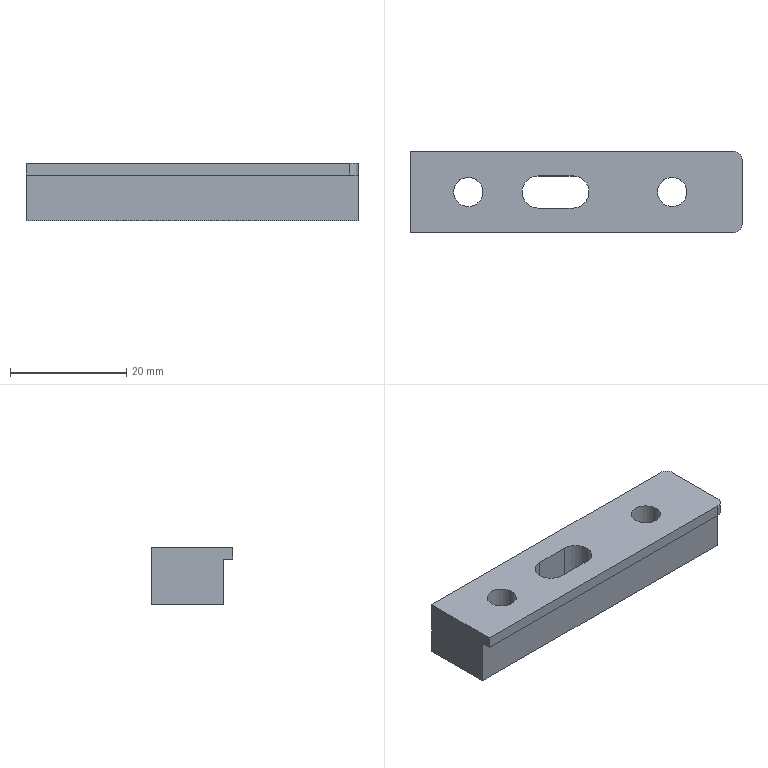Part | STEP file | 200 mesh_id6_xmt_t | 1 solid | 16 faces | box 57 x 14 x 9.8 mm | volume 6159 mm3 | plane 10 | cylinder 6 | commonest cylinder face diameters 3 x2 5.02 x2 5.5 x2
STEP:
#1=CARTESIAN_POINT('',(-16856.158,-3972.269,52.7));
#2=VERTEX_POINT('',#1);
#3=CARTESIAN_POINT('',(-16853.648,-3972.269,52.7));
#4=DIRECTION('',(0.,0.,-1.));
#5=DIRECTION('',(-1.,0.,0.));
#6=AXIS2_PLACEMENT_3D('',#3,#4,#5);
#7=CIRCLE('',#6,2.51);
#8=EDGE_CURVE('',#2,#2,#7,.T.);
#9=ORIENTED_EDGE('',*,*,#8,.T.);
#10=EDGE_LOOP('',(#9));
#11=FACE_BOUND('',#10,.T.);
#12=CARTESIAN_POINT('',(-16891.158,-3972.269,52.7));
#13=VERTEX_POINT('',#12);
#14=CARTESIAN_POINT('',(-16888.648,-3972.269,52.7));
#15=DIRECTION('',(0.,0.,-1.));
#16=DIRECTION('',(-1.,0.,0.));
#17=AXIS2_PLACEMENT_3D('',#14,#15,#16);
#18=CIRCLE('',#17,2.51);
#19=EDGE_CURVE('',#13,#13,#18,.T.);
#20=ORIENTED_EDGE('',*,*,#19,.T.);
#21=EDGE_LOOP('',(#20));
#22=FACE_BOUND('',#21,.T.);
#23=CARTESIAN_POINT('',(-16898.648,-3965.269,52.7));
#24=VERTEX_POINT('',#23);
#25=CARTESIAN_POINT('',(-16843.148,-3965.269,52.7));
#26=VERTEX_POINT('',#25);
#27=CARTESIAN_POINT('',(-16897.148,-3965.269,52.7));
#28=DIRECTION('',(1.,0.,0.));
#29=VECTOR('',#28,1.);
#30=LINE('',#27,#29);
#31=EDGE_CURVE('',#24,#26,#30,.T.);
#32=ORIENTED_EDGE('',*,*,#31,.F.);
#33=CARTESIAN_POINT('',(-16898.648,-3979.269,52.7));
#34=VERTEX_POINT('',#33);
#35=CARTESIAN_POINT('',(-16898.648,-3977.769,52.7));
#36=DIRECTION('',(0.,1.,0.));
#37=VECTOR('',#36,1.);
#38=LINE('',#35,#37);
#39=EDGE_CURVE('',#34,#24,#38,.T.);
#40=ORIENTED_EDGE('',*,*,#39,.F.);
#41=CARTESIAN_POINT('',(-16843.148,-3979.269,52.7));
#42=VERTEX_POINT('',#41);
#43=CARTESIAN_POINT('',(-16843.148,-3979.269,52.7));
#44=DIRECTION('',(-1.,0.,0.));
#45=VECTOR('',#44,1.);
#46=LINE('',#43,#45);
#47=EDGE_CURVE('',#42,#34,#46,.T.);
#48=ORIENTED_EDGE('',*,*,#47,.F.);
#49=CARTESIAN_POINT('',(-16841.648,-3977.769,52.7));
#50=VERTEX_POINT('',#49);
#51=CARTESIAN_POINT('',(-16843.148,-3977.769,52.7));
#52=DIRECTION('',(0.,0.,-1.));
#53=DIRECTION('',(1.,0.,0.));
#54=AXIS2_PLACEMENT_3D('',#51,#52,#53);
#55=CIRCLE('',#54,1.5);
#56=EDGE_CURVE('',#50,#42,#55,.T.);
#57=ORIENTED_EDGE('',*,*,#56,.F.);
#58=CARTESIAN_POINT('',(-16841.648,-3966.769,52.7));
#59=VERTEX_POINT('',#58);
#60=CARTESIAN_POINT('',(-16841.648,-3968.769,52.7));
#61=DIRECTION('',(0.,-1.,0.));
#62=VECTOR('',#61,1.);
#63=LINE('',#60,#62);
#64=EDGE_CURVE('',#59,#50,#63,.T.);
#65=ORIENTED_EDGE('',*,*,#64,.F.);
#66=CARTESIAN_POINT('',(-16843.148,-3966.769,52.7));
#67=DIRECTION('',(0.,0.,-1.));
#68=DIRECTION('',(-1.,0.,0.));
#69=AXIS2_PLACEMENT_3D('',#66,#67,#68);
#70=CIRCLE('',#69,1.5);
#71=EDGE_CURVE('',#26,#59,#70,.T.);
#72=ORIENTED_EDGE('',*,*,#71,.F.);
#73=EDGE_LOOP('',(#32,#40,#48,#57,#65,#72));
#74=FACE_BOUND('',#73,.T.);
#75=CARTESIAN_POINT('',(-16876.648,-3975.019,52.7));
#76=VERTEX_POINT('',#75);
#77=CARTESIAN_POINT('',(-16870.648,-3975.019,52.7));
#78=VERTEX_POINT('',#77);
#79=CARTESIAN_POINT('',(-16873.648,-3975.019,52.7));
#80=DIRECTION('',(1.,0.,0.));
#81=VECTOR('',#80,1.);
#82=LINE('',#79,#81);
#83=EDGE_CURVE('',#76,#78,#82,.T.);
#84=ORIENTED_EDGE('',*,*,#83,.F.);
#85=CARTESIAN_POINT('',(-16876.648,-3969.519,52.7));
#86=VERTEX_POINT('',#85);
#87=CARTESIAN_POINT('',(-16876.648,-3972.269,52.7));
#88=DIRECTION('',(0.,0.,1.));
#89=DIRECTION('',(-1.,0.,0.));
#90=AXIS2_PLACEMENT_3D('',#87,#88,#89);
#91=CIRCLE('',#90,2.75);
#92=EDGE_CURVE('',#86,#76,#91,.T.);
#93=ORIENTED_EDGE('',*,*,#92,.F.);
#94=CARTESIAN_POINT('',(-16870.648,-3969.519,52.7));
#95=VERTEX_POINT('',#94);
#96=CARTESIAN_POINT('',(-16873.648,-3969.519,52.7));
#97=DIRECTION('',(-1.,0.,0.));
#98=VECTOR('',#97,1.);
#99=LINE('',#96,#98);
#100=EDGE_CURVE('',#95,#86,#99,.T.);
#101=ORIENTED_EDGE('',*,*,#100,.F.);
#102=CARTESIAN_POINT('',(-16870.648,-3972.269,52.7));
#103=DIRECTION('',(0.,0.,1.));
#104=DIRECTION('',(1.,0.,0.));
#105=AXIS2_PLACEMENT_3D('',#102,#103,#104);
#106=CIRCLE('',#105,2.75);
#107=EDGE_CURVE('',#78,#95,#106,.T.);
#108=ORIENTED_EDGE('',*,*,#107,.F.);
#109=EDGE_LOOP('',(#84,#93,#101,#108));
#110=FACE_BOUND('',#109,.T.);
#111=CARTESIAN_POINT('',(-16897.148,-3968.769,52.7));
#112=DIRECTION('',(0.,0.,-1.));
#113=DIRECTION('',(-1.,0.,0.));
#114=AXIS2_PLACEMENT_3D('',#111,#112,#113);
#115=PLANE('',#114);
#116=ADVANCED_FACE('',(#11,#22,#74,#110),#115,.F.);
#117=CARTESIAN_POINT('',(-16898.648,-3965.269,42.9));
#118=VERTEX_POINT('',#117);
#119=CARTESIAN_POINT('',(-16898.648,-3965.269,40.7));
#120=DIRECTION('',(0.,0.,1.));
#121=VECTOR('',#120,1.);
#122=LINE('',#119,#121);
#123=EDGE_CURVE('',#118,#24,#122,.T.);
#124=ORIENTED_EDGE('',*,*,#123,.F.);
#125=CARTESIAN_POINT('',(-16898.648,-3977.669,42.9));
#126=VERTEX_POINT('',#125);
#127=CARTESIAN_POINT('',(-16898.648,-3968.769,42.9));
#128=DIRECTION('',(0.,1.,0.));
#129=VECTOR('',#128,1.);
#130=LINE('',#127,#129);
#131=EDGE_CURVE('',#126,#118,#130,.T.);
#132=ORIENTED_EDGE('',*,*,#131,.F.);
#133=CARTESIAN_POINT('',(-16898.648,-3977.669,50.7));
#134=VERTEX_POINT('',#133);
#135=CARTESIAN_POINT('',(-16898.648,-3977.669,40.7));
#136=DIRECTION('',(0.,0.,-1.));
#137=VECTOR('',#136,1.);
#138=LINE('',#135,#137);
#139=EDGE_CURVE('',#134,#126,#138,.T.);
#140=ORIENTED_EDGE('',*,*,#139,.F.);
#141=CARTESIAN_POINT('',(-16898.648,-3979.269,50.7));
#142=VERTEX_POINT('',#141);
#143=CARTESIAN_POINT('',(-16898.648,-3977.769,50.7));
#144=DIRECTION('',(0.,1.,0.));
#145=VECTOR('',#144,1.);
#146=LINE('',#143,#145);
#147=EDGE_CURVE('',#142,#134,#146,.T.);
#148=ORIENTED_EDGE('',*,*,#147,.F.);
#149=CARTESIAN_POINT('',(-16898.648,-3979.269,40.7));
#150=DIRECTION('',(0.,0.,1.));
#151=VECTOR('',#150,1.);
#152=LINE('',#149,#151);
#153=EDGE_CURVE('',#142,#34,#152,.T.);
#154=ORIENTED_EDGE('',*,*,#153,.T.);
#155=ORIENTED_EDGE('',*,*,#39,.T.);
#156=EDGE_LOOP('',(#124,#132,#140,#148,#154,#155));
#157=FACE_OUTER_BOUND('',#156,.T.);
#158=CARTESIAN_POINT('',(-16898.648,-3977.769,40.7));
#159=DIRECTION('',(1.,0.,0.));
#160=DIRECTION('',(0.,0.,-1.));
#161=AXIS2_PLACEMENT_3D('',#158,#159,#160);
#162=PLANE('',#161);
#163=ADVANCED_FACE('',(#157),#162,.F.);
#164=CARTESIAN_POINT('',(-16876.648,-3975.019,42.9));
#165=VERTEX_POINT('',#164);
#166=CARTESIAN_POINT('',(-16876.648,-3969.519,42.9));
#167=VERTEX_POINT('',#166);
#168=CARTESIAN_POINT('',(-16876.648,-3972.269,42.9));
#169=DIRECTION('',(0.,0.,-1.));
#170=DIRECTION('',(-1.,0.,0.));
#171=AXIS2_PLACEMENT_3D('',#168,#169,#170);
#172=CIRCLE('',#171,2.75);
#173=EDGE_CURVE('',#165,#167,#172,.T.);
#174=ORIENTED_EDGE('',*,*,#173,.F.);
#175=CARTESIAN_POINT('',(-16870.648,-3975.019,42.9));
#176=VERTEX_POINT('',#175);
#177=CARTESIAN_POINT('',(-16897.148,-3975.019,42.9));
#178=DIRECTION('',(-1.,0.,0.));
#179=VECTOR('',#178,1.);
#180=LINE('',#177,#179);
#181=EDGE_CURVE('',#176,#165,#180,.T.);
#182=ORIENTED_EDGE('',*,*,#181,.F.);
#183=CARTESIAN_POINT('',(-16870.648,-3969.519,42.9));
#184=VERTEX_POINT('',#183);
#185=CARTESIAN_POINT('',(-16870.648,-3972.269,42.9));
#186=DIRECTION('',(0.,0.,-1.));
#187=DIRECTION('',(-1.,0.,0.));
#188=AXIS2_PLACEMENT_3D('',#185,#186,#187);
#189=CIRCLE('',#188,2.75);
#190=EDGE_CURVE('',#184,#176,#189,.T.);
#191=ORIENTED_EDGE('',*,*,#190,.F.);
#192=CARTESIAN_POINT('',(-16897.148,-3969.519,42.9));
#193=DIRECTION('',(1.,0.,0.));
#194=VECTOR('',#193,1.);
#195=LINE('',#192,#194);
#196=EDGE_CURVE('',#167,#184,#195,.T.);
#197=ORIENTED_EDGE('',*,*,#196,.F.);
#198=EDGE_LOOP('',(#174,#182,#191,#197));
#199=FACE_BOUND('',#198,.T.);
#200=CARTESIAN_POINT('',(-16851.138,-3972.269,42.9));
#201=VERTEX_POINT('',#200);
#202=CARTESIAN_POINT('',(-16853.648,-3972.269,42.9));
#203=DIRECTION('',(0.,0.,1.));
#204=DIRECTION('',(1.,0.,0.));
#205=AXIS2_PLACEMENT_3D('',#202,#203,#204);
#206=CIRCLE('',#205,2.51);
#207=EDGE_CURVE('',#201,#201,#206,.T.);
#208=ORIENTED_EDGE('',*,*,#207,.T.);
#209=EDGE_LOOP('',(#208));
#210=FACE_BOUND('',#209,.T.);
#211=CARTESIAN_POINT('',(-16886.138,-3972.269,42.9));
#212=VERTEX_POINT('',#211);
#213=CARTESIAN_POINT('',(-16888.648,-3972.269,42.9));
#214=DIRECTION('',(0.,0.,1.));
#215=DIRECTION('',(1.,0.,0.));
#216=AXIS2_PLACEMENT_3D('',#213,#214,#215);
#217=CIRCLE('',#216,2.51);
#218=EDGE_CURVE('',#212,#212,#217,.T.);
#219=ORIENTED_EDGE('',*,*,#218,.T.);
#220=EDGE_LOOP('',(#219));
#221=FACE_BOUND('',#220,.T.);
#222=CARTESIAN_POINT('',(-16841.648,-3977.669,42.9));
#223=VERTEX_POINT('',#222);
#224=CARTESIAN_POINT('',(-16898.648,-3977.669,42.9));
#225=DIRECTION('',(1.,0.,0.));
#226=VECTOR('',#225,1.);
#227=LINE('',#224,#226);
#228=EDGE_CURVE('',#126,#223,#227,.T.);
#229=ORIENTED_EDGE('',*,*,#228,.F.);
#230=ORIENTED_EDGE('',*,*,#131,.T.);
#231=CARTESIAN_POINT('',(-16843.148,-3965.269,42.9));
#232=VERTEX_POINT('',#231);
#233=CARTESIAN_POINT('',(-16897.148,-3965.269,42.9));
#234=DIRECTION('',(1.,0.,0.));
#235=VECTOR('',#234,1.);
#236=LINE('',#233,#235);
#237=EDGE_CURVE('',#118,#232,#236,.T.);
#238=ORIENTED_EDGE('',*,*,#237,.T.);
#239=CARTESIAN_POINT('',(-16841.648,-3966.769,42.9));
#240=VERTEX_POINT('',#239);
#241=CARTESIAN_POINT('',(-16843.148,-3966.769,42.9));
#242=DIRECTION('',(0.,0.,-1.));
#243=DIRECTION('',(-1.,0.,0.));
#244=AXIS2_PLACEMENT_3D('',#241,#242,#243);
#245=CIRCLE('',#244,1.5);
#246=EDGE_CURVE('',#232,#240,#245,.T.);
#247=ORIENTED_EDGE('',*,*,#246,.T.);
#248=CARTESIAN_POINT('',(-16841.648,-3968.769,42.9));
#249=DIRECTION('',(0.,-1.,0.));
#250=VECTOR('',#249,1.);
#251=LINE('',#248,#250);
#252=EDGE_CURVE('',#240,#223,#251,.T.);
#253=ORIENTED_EDGE('',*,*,#252,.T.);
#254=EDGE_LOOP('',(#229,#230,#238,#247,#253));
#255=FACE_BOUND('',#254,.T.);
#256=CARTESIAN_POINT('',(-16897.148,-3968.769,42.9));
#257=DIRECTION('',(0.,0.,-1.));
#258=DIRECTION('',(-1.,0.,0.));
#259=AXIS2_PLACEMENT_3D('',#256,#257,#258);
#260=PLANE('',#259);
#261=ADVANCED_FACE('',(#199,#210,#221,#255),#260,.T.);
#262=CARTESIAN_POINT('',(-16841.648,-3977.669,50.7));
#263=VERTEX_POINT('',#262);
#264=CARTESIAN_POINT('',(-16841.648,-3977.669,40.7));
#265=DIRECTION('',(0.,0.,1.));
#266=VECTOR('',#265,1.);
#267=LINE('',#264,#266);
#268=EDGE_CURVE('',#223,#263,#267,.T.);
#269=ORIENTED_EDGE('',*,*,#268,.F.);
#270=ORIENTED_EDGE('',*,*,#252,.F.);
#271=CARTESIAN_POINT('',(-16841.648,-3966.769,40.7));
#272=DIRECTION('',(0.,0.,1.));
#273=VECTOR('',#272,1.);
#274=LINE('',#271,#273);
#275=EDGE_CURVE('',#240,#59,#274,.T.);
#276=ORIENTED_EDGE('',*,*,#275,.T.);
#277=ORIENTED_EDGE('',*,*,#64,.T.);
#278=CARTESIAN_POINT('',(-16841.648,-3977.769,50.7));
#279=VERTEX_POINT('',#278);
#280=CARTESIAN_POINT('',(-16841.648,-3977.769,40.7));
#281=DIRECTION('',(0.,0.,1.));
#282=VECTOR('',#281,1.);
#283=LINE('',#280,#282);
#284=EDGE_CURVE('',#279,#50,#283,.T.);
#285=ORIENTED_EDGE('',*,*,#284,.F.);
#286=CARTESIAN_POINT('',(-16841.648,-3968.769,50.7));
#287=DIRECTION('',(0.,-1.,0.));
#288=VECTOR('',#287,1.);
#289=LINE('',#286,#288);
#290=EDGE_CURVE('',#263,#279,#289,.T.);
#291=ORIENTED_EDGE('',*,*,#290,.F.);
#292=EDGE_LOOP('',(#269,#270,#276,#277,#285,#291));
#293=FACE_OUTER_BOUND('',#292,.T.);
#294=CARTESIAN_POINT('',(-16841.648,-3968.769,40.7));
#295=DIRECTION('',(-1.,0.,0.));
#296=DIRECTION('',(0.,0.,1.));
#297=AXIS2_PLACEMENT_3D('',#294,#295,#296);
#298=PLANE('',#297);
#299=ADVANCED_FACE('',(#293),#298,.F.);
#300=CARTESIAN_POINT('',(-16843.148,-3979.269,50.7));
#301=VERTEX_POINT('',#300);
#302=CARTESIAN_POINT('',(-16843.148,-3977.769,50.7));
#303=DIRECTION('',(0.,0.,-1.));
#304=DIRECTION('',(-1.,0.,0.));
#305=AXIS2_PLACEMENT_3D('',#302,#303,#304);
#306=CIRCLE('',#305,1.5);
#307=EDGE_CURVE('',#279,#301,#306,.T.);
#308=ORIENTED_EDGE('',*,*,#307,.F.);
#309=ORIENTED_EDGE('',*,*,#284,.T.);
#310=ORIENTED_EDGE('',*,*,#56,.T.);
#311=CARTESIAN_POINT('',(-16843.148,-3979.269,40.7));
#312=DIRECTION('',(0.,0.,1.));
#313=VECTOR('',#312,1.);
#314=LINE('',#311,#313);
#315=EDGE_CURVE('',#301,#42,#314,.T.);
#316=ORIENTED_EDGE('',*,*,#315,.F.);
#317=EDGE_LOOP('',(#308,#309,#310,#316));
#318=FACE_OUTER_BOUND('',#317,.T.);
#319=CARTESIAN_POINT('',(-16843.148,-3977.769,40.7));
#320=DIRECTION('',(0.,0.,1.));
#321=DIRECTION('',(1.,0.,0.));
#322=AXIS2_PLACEMENT_3D('',#319,#320,#321);
#323=CYLINDRICAL_SURFACE('',#322,1.5);
#324=ADVANCED_FACE('',(#318),#323,.T.);
#325=ORIENTED_EDGE('',*,*,#153,.F.);
#326=CARTESIAN_POINT('',(-16843.148,-3979.269,50.7));
#327=DIRECTION('',(-1.,0.,0.));
#328=VECTOR('',#327,1.);
#329=LINE('',#326,#328);
#330=EDGE_CURVE('',#301,#142,#329,.T.);
#331=ORIENTED_EDGE('',*,*,#330,.F.);
#332=ORIENTED_EDGE('',*,*,#315,.T.);
#333=ORIENTED_EDGE('',*,*,#47,.T.);
#334=EDGE_LOOP('',(#325,#331,#332,#333));
#335=FACE_OUTER_BOUND('',#334,.T.);
#336=CARTESIAN_POINT('',(-16843.148,-3979.269,40.7));
#337=DIRECTION('',(0.,1.,0.));
#338=DIRECTION('',(0.,0.,1.));
#339=AXIS2_PLACEMENT_3D('',#336,#337,#338);
#340=PLANE('',#339);
#341=ADVANCED_FACE('',(#335),#340,.F.);
#342=ORIENTED_EDGE('',*,*,#237,.F.);
#343=ORIENTED_EDGE('',*,*,#123,.T.);
#344=ORIENTED_EDGE('',*,*,#31,.T.);
#345=CARTESIAN_POINT('',(-16843.148,-3965.269,40.7));
#346=DIRECTION('',(0.,0.,1.));
#347=VECTOR('',#346,1.);
#348=LINE('',#345,#347);
#349=EDGE_CURVE('',#232,#26,#348,.T.);
#350=ORIENTED_EDGE('',*,*,#349,.F.);
#351=EDGE_LOOP('',(#342,#343,#344,#350));
#352=FACE_OUTER_BOUND('',#351,.T.);
#353=CARTESIAN_POINT('',(-16897.148,-3965.269,40.7));
#354=DIRECTION('',(0.,-1.,0.));
#355=DIRECTION('',(0.,0.,-1.));
#356=AXIS2_PLACEMENT_3D('',#353,#354,#355);
#357=PLANE('',#356);
#358=ADVANCED_FACE('',(#352),#357,.F.);
#359=ORIENTED_EDGE('',*,*,#349,.T.);
#360=ORIENTED_EDGE('',*,*,#71,.T.);
#361=ORIENTED_EDGE('',*,*,#275,.F.);
#362=ORIENTED_EDGE('',*,*,#246,.F.);
#363=EDGE_LOOP('',(#359,#360,#361,#362));
#364=FACE_OUTER_BOUND('',#363,.T.);
#365=CARTESIAN_POINT('',(-16843.148,-3966.769,40.7));
#366=DIRECTION('',(0.,0.,1.));
#367=DIRECTION('',(1.,0.,0.));
#368=AXIS2_PLACEMENT_3D('',#365,#366,#367);
#369=CYLINDRICAL_SURFACE('',#368,1.5);
#370=ADVANCED_FACE('',(#364),#369,.T.);
#371=ORIENTED_EDGE('',*,*,#139,.T.);
#372=ORIENTED_EDGE('',*,*,#228,.T.);
#373=ORIENTED_EDGE('',*,*,#268,.T.);
#374=CARTESIAN_POINT('',(-16898.648,-3977.669,50.7));
#375=DIRECTION('',(1.,0.,0.));
#376=VECTOR('',#375,1.);
#377=LINE('',#374,#376);
#378=EDGE_CURVE('',#134,#263,#377,.T.);
#379=ORIENTED_EDGE('',*,*,#378,.F.);
#380=EDGE_LOOP('',(#371,#372,#373,#379));
#381=FACE_OUTER_BOUND('',#380,.T.);
#382=CARTESIAN_POINT('',(-16898.648,-3977.669,50.7));
#383=DIRECTION('',(0.,-1.,0.));
#384=DIRECTION('',(1.,0.,0.));
#385=AXIS2_PLACEMENT_3D('',#382,#383,#384);
#386=PLANE('',#385);
#387=ADVANCED_FACE('',(#381),#386,.T.);
#388=ORIENTED_EDGE('',*,*,#330,.T.);
#389=ORIENTED_EDGE('',*,*,#147,.T.);
#390=ORIENTED_EDGE('',*,*,#378,.T.);
#391=ORIENTED_EDGE('',*,*,#290,.T.);
#392=ORIENTED_EDGE('',*,*,#307,.T.);
#393=EDGE_LOOP('',(#388,#389,#390,#391,#392));
#394=FACE_OUTER_BOUND('',#393,.T.);
#395=CARTESIAN_POINT('',(-16898.648,-3979.269,50.7));
#396=DIRECTION('',(0.,0.,-1.));
#397=DIRECTION('',(-1.,0.,0.));
#398=AXIS2_PLACEMENT_3D('',#395,#396,#397);
#399=PLANE('',#398);
#400=ADVANCED_FACE('',(#394),#399,.T.);
#401=ORIENTED_EDGE('',*,*,#218,.F.);
#402=EDGE_LOOP('',(#401));
#403=FACE_BOUND('',#402,.T.);
#404=ORIENTED_EDGE('',*,*,#19,.F.);
#405=EDGE_LOOP('',(#404));
#406=FACE_BOUND('',#405,.T.);
#407=CARTESIAN_POINT('',(-16888.648,-3972.269,42.9));
#408=DIRECTION('',(0.,0.,1.));
#409=DIRECTION('',(1.,0.,0.));
#410=AXIS2_PLACEMENT_3D('',#407,#408,#409);
#411=CYLINDRICAL_SURFACE('',#410,2.51);
#412=ADVANCED_FACE('',(#403,#406),#411,.F.);
#413=ORIENTED_EDGE('',*,*,#207,.F.);
#414=EDGE_LOOP('',(#413));
#415=FACE_BOUND('',#414,.T.);
#416=ORIENTED_EDGE('',*,*,#8,.F.);
#417=EDGE_LOOP('',(#416));
#418=FACE_BOUND('',#417,.T.);
#419=CARTESIAN_POINT('',(-16853.648,-3972.269,42.9));
#420=DIRECTION('',(0.,0.,1.));
#421=DIRECTION('',(1.,0.,0.));
#422=AXIS2_PLACEMENT_3D('',#419,#420,#421);
#423=CYLINDRICAL_SURFACE('',#422,2.51);
#424=ADVANCED_FACE('',(#415,#418),#423,.F.);
#425=ORIENTED_EDGE('',*,*,#181,.T.);
#426=CARTESIAN_POINT('',(-16876.648,-3975.019,28.2));
#427=DIRECTION('',(0.,0.,-1.));
#428=VECTOR('',#427,1.);
#429=LINE('',#426,#428);
#430=EDGE_CURVE('',#76,#165,#429,.T.);
#431=ORIENTED_EDGE('',*,*,#430,.F.);
#432=ORIENTED_EDGE('',*,*,#83,.T.);
#433=CARTESIAN_POINT('',(-16870.648,-3975.019,28.2));
#434=DIRECTION('',(0.,0.,-1.));
#435=VECTOR('',#434,1.);
#436=LINE('',#433,#435);
#437=EDGE_CURVE('',#78,#176,#436,.T.);
#438=ORIENTED_EDGE('',*,*,#437,.T.);
#439=EDGE_LOOP('',(#425,#431,#432,#438));
#440=FACE_OUTER_BOUND('',#439,.T.);
#441=CARTESIAN_POINT('',(-16873.648,-3975.019,28.2));
#442=DIRECTION('',(0.,-1.,0.));
#443=DIRECTION('',(0.,0.,-1.));
#444=AXIS2_PLACEMENT_3D('',#441,#442,#443);
#445=PLANE('',#444);
#446=ADVANCED_FACE('',(#440),#445,.F.);
#447=ORIENTED_EDGE('',*,*,#196,.T.);
#448=CARTESIAN_POINT('',(-16870.648,-3969.519,28.2));
#449=DIRECTION('',(0.,0.,-1.));
#450=VECTOR('',#449,1.);
#451=LINE('',#448,#450);
#452=EDGE_CURVE('',#95,#184,#451,.T.);
#453=ORIENTED_EDGE('',*,*,#452,.F.);
#454=ORIENTED_EDGE('',*,*,#100,.T.);
#455=CARTESIAN_POINT('',(-16876.648,-3969.519,28.2));
#456=DIRECTION('',(0.,0.,-1.));
#457=VECTOR('',#456,1.);
#458=LINE('',#455,#457);
#459=EDGE_CURVE('',#86,#167,#458,.T.);
#460=ORIENTED_EDGE('',*,*,#459,.T.);
#461=EDGE_LOOP('',(#447,#453,#454,#460));
#462=FACE_OUTER_BOUND('',#461,.T.);
#463=CARTESIAN_POINT('',(-16873.648,-3969.519,28.2));
#464=DIRECTION('',(0.,1.,0.));
#465=DIRECTION('',(0.,0.,1.));
#466=AXIS2_PLACEMENT_3D('',#463,#464,#465);
#467=PLANE('',#466);
#468=ADVANCED_FACE('',(#462),#467,.F.);
#469=ORIENTED_EDGE('',*,*,#173,.T.);
#470=ORIENTED_EDGE('',*,*,#459,.F.);
#471=ORIENTED_EDGE('',*,*,#92,.T.);
#472=ORIENTED_EDGE('',*,*,#430,.T.);
#473=EDGE_LOOP('',(#469,#470,#471,#472));
#474=FACE_OUTER_BOUND('',#473,.T.);
#475=CARTESIAN_POINT('',(-16876.648,-3972.269,28.2));
#476=DIRECTION('',(0.,0.,1.));
#477=DIRECTION('',(1.,0.,0.));
#478=AXIS2_PLACEMENT_3D('',#475,#476,#477);
#479=CYLINDRICAL_SURFACE('',#478,2.75);
#480=ADVANCED_FACE('',(#474),#479,.F.);
#481=ORIENTED_EDGE('',*,*,#190,.T.);
#482=ORIENTED_EDGE('',*,*,#437,.F.);
#483=ORIENTED_EDGE('',*,*,#107,.T.);
#484=ORIENTED_EDGE('',*,*,#452,.T.);
#485=EDGE_LOOP('',(#481,#482,#483,#484));
#486=FACE_OUTER_BOUND('',#485,.T.);
#487=CARTESIAN_POINT('',(-16870.648,-3972.269,28.2));
#488=DIRECTION('',(0.,0.,1.));
#489=DIRECTION('',(1.,0.,0.));
#490=AXIS2_PLACEMENT_3D('',#487,#488,#489);
#491=CYLINDRICAL_SURFACE('',#490,2.75);
#492=ADVANCED_FACE('',(#486),#491,.F.);
#493=CLOSED_SHELL('',(#116,#163,#261,#299,#324,#341,#358,#370,#387,#400,#412,#424,#446,#468,#480,#492));
#494=MANIFOLD_SOLID_BREP('',#493);
#495=(LENGTH_UNIT()NAMED_UNIT(*)SI_UNIT(.MILLI.,.METRE.));
#496=UNCERTAINTY_MEASURE_WITH_UNIT(LENGTH_MEASURE(0.00002),#495,'','');
#497=(NAMED_UNIT(*)PLANE_ANGLE_UNIT()SI_UNIT($,.RADIAN.));
#498=PLANE_ANGLE_MEASURE_WITH_UNIT(PLANE_ANGLE_MEASURE(0.01745),#497);
#499=DIMENSIONAL_EXPONENTS(0.,0.,0.,0.,0.,0.,0.);
#500=(CONVERSION_BASED_UNIT('DEGREE',#498)NAMED_UNIT(#499)PLANE_ANGLE_UNIT());
#501=(NAMED_UNIT(*)SI_UNIT($,.STERADIAN.)SOLID_ANGLE_UNIT());
#502=(GEOMETRIC_REPRESENTATION_CONTEXT(3)GLOBAL_UNCERTAINTY_ASSIGNED_CONTEXT((#496))GLOBAL_UNIT_ASSIGNED_CONTEXT((#495,#500,#501))REPRESENTATION_CONTEXT('',''));
#503=ADVANCED_BREP_SHAPE_REPRESENTATION('',(#494),#502);